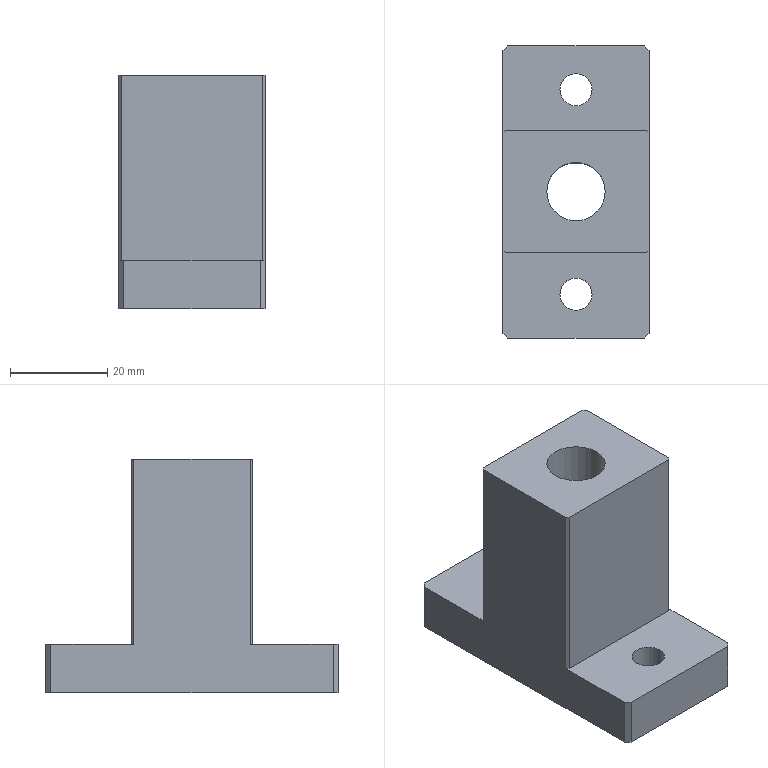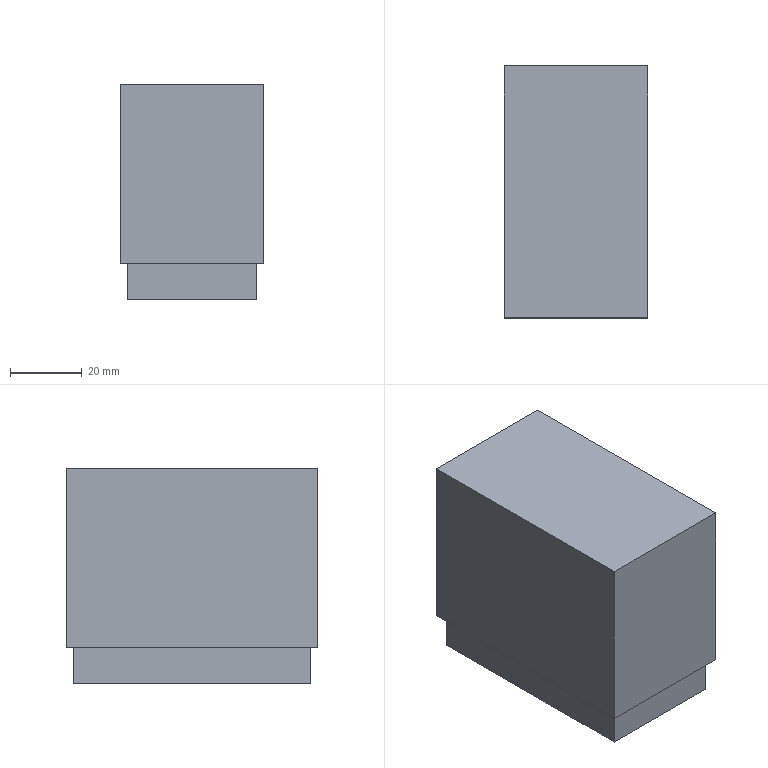CAM job | NX | 3-axis milling, drilling | part box 30 x 60 x 48 mm | stock box 40 x 70 x 60 mm
Tools:
number,name,description,diameter,corner_radius,flute_length,length,flutes
1,D50面刀,,50.0,0.0,50.0,75.0,2
2,D16开粗,,16.0,0.0,50.0,75.0,2
3,D16精光,,16.0,0.0,50.0,75.0,2
5,D6倒角刀,,6.0,0.0,50.0,75.0,2
10,D10.4钻头,,10.4,0.0,35.0,50.0,2
12,D7钻头,,7.0,0.0,35.0,50.0,2
11,M12,,12.0,0.0,35.0,50.0,2
Operations:
program,operation,operation_type,tool,method,geometry_group,spindle_rpm,surface_speed,feed_per_tooth,feed_cut,feed_plunge,cut_length_mm,path_length_mm,cut_time_min,machine_time_min
G54,PLANAR_MILL,PlanarMilling,D50面刀,METHOD,WORKPIECE,1600.0,251.0,0.25,800.0,100.0,124.0,158.0,0.155,0.1584
G54,ADAPTIVE_MILLING,CavityMilling,D16开粗,METHOD,WORKPIECE,4500.0,226.0,0.2222,2000.0,100.0,21664.99,22230.747,7.077,7.134
G54,PLANAR_MILL_1,PlanarMilling,D16精光,METHOD,WORKPIECE,2800.0,140.0,0.1071,600.0,100.0,293.722,892.871,0.4895,0.5495
G54,PLANAR_MILL_1_COPY,PlanarMilling,D16精光,METHOD,WORKPIECE,2800.0,140.0,0.1071,600.0,100.0,275.922,858.135,0.4599,0.5181
G54,PLANAR_MILL_2,PlanarMilling,D16精光,METHOD,WORKPIECE,2800.0,140.0,0.1071,600.0,100.0,978.955,1434.498,1.632,1.677
G54,DRILLING,Operation,D6倒角刀,METHOD,WORKPIECE,1600.0,30.0,0.0187,60.0,0.0,5.0,50.0,0.0833,0.0878
G54,DRILLING_COPY_1,Operation,D6倒角刀,METHOD,WORKPIECE,1600.0,30.0,0.0187,60.0,0.0,10.0,181.107,0.1667,0.1838
G54,DRILLING_COPY,Operation,D10.4钻头,METHOD,WORKPIECE,600.0,19.0,0.025,30.0,0.0,55.0,150.0,1.833,1.843
G54,DRILLING_COPY_1_COPY,Operation,D7钻头,METHOD,WORKPIECE,1600.0,30.0,0.0187,60.0,0.0,34.0,229.107,0.5667,0.5862
G54,PLANAR_MILL_3,PlanarMilling,D6倒角刀,METHOD,WORKPIECE,3000.0,56.0,0.1333,800.0,100.0,131.678,171.678,0.1646,0.1686
G54,PLANAR_MILL_3_COPY_COPY,PlanarMilling,D6倒角刀,METHOD,WORKPIECE,3000.0,56.0,0.1333,800.0,100.0,33.852,73.852,0.0423,0.0463
G54,PLANAR_MILL_3_COPY_COPY_1,PlanarMilling,D6倒角刀,METHOD,WORKPIECE,3000.0,56.0,0.1333,800.0,100.0,22.619,302.62,0.0283,0.0563
G54,PLANAR_MILL_3_COPY,PlanarMilling,D6倒角刀,METHOD,WORKPIECE,3000.0,56.0,0.1333,800.0,100.0,126.282,394.682,0.1579,0.1847
G54,DRILLING_COPY_COPY,Operation,M12,METHOD,WORKPIECE,200.0,7.0,0.0044,1.75,0.0,8.0,56.0,4.571,4.576
G55,ADAPTIVE_MILLING_1,CavityMilling,D16开粗,METHOD,WORKPIECE_1,3500.0,175.0,0.2857,2000.0,100.0,9389.707,9423.507,4.695,4.698
G55,PLANAR_MILL_4,PlanarMilling,D50面刀,METHOD,WORKPIECE_1,1600.0,251.0,0.1875,600.0,100.0,120.0,154.0,0.2,0.2034
G55,PLANAR_MILL_5,PlanarMilling,D6倒角刀,METHOD,WORKPIECE_1,3000.0,56.0,0.1667,1000.0,100.0,202.223,240.223,0.2022,0.206
G55,PLANAR_MILL_5_COPY,PlanarMilling,D6倒角刀,METHOD,WORKPIECE_1,3000.0,56.0,0.1667,1000.0,100.0,66.213,226.018,0.0662,0.0822